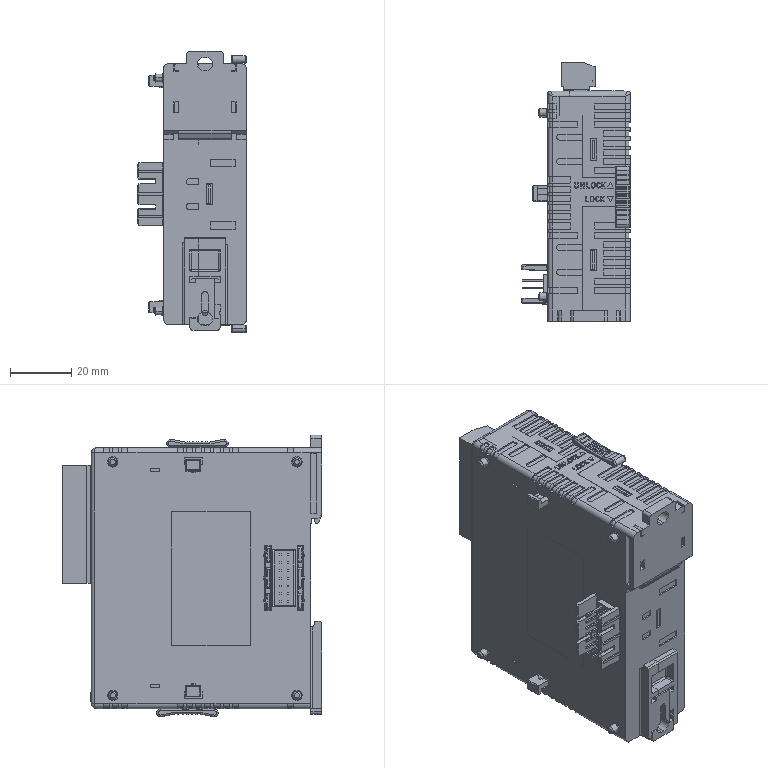Part | SolidWorks | features BaseBody 1 | 1 solid | 3789 faces | volume 162507 mm3 | plane 2698 | cylinder 970 | cone 60 | spline 31 | torus 26 | sphere 4 | commonest cylinder face diameters 0.4 x624 1 x70 2.4 x66 3.4 x62 0.6 x37 2.6 x33